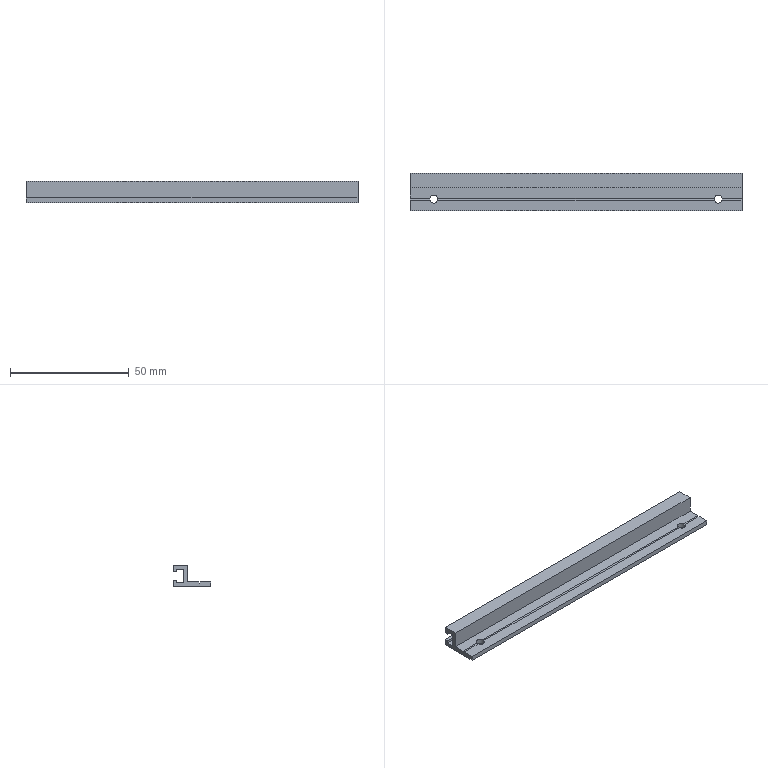Part | STEP file | 0230_016_SENBF3-140 | 1 solid | 27 faces | box 140 x 16 x 9 mm | volume 7179 mm3 | plane 23 | cylinder 4 | commonest cylinder face diameters 3.5 x4